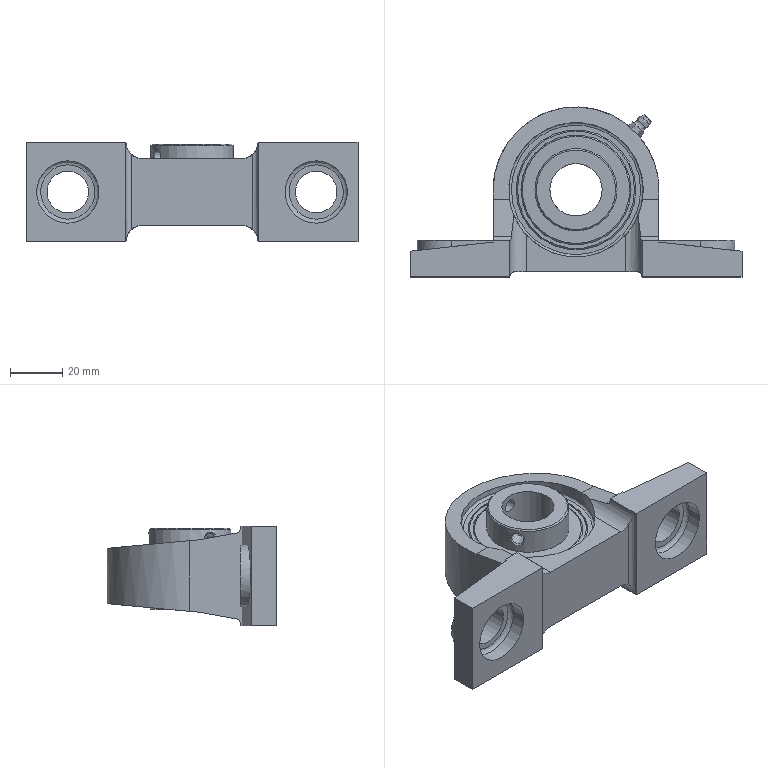Part | STEP file | Pillow block bearing UCP204_D20 | 1 solid | 92 faces | box 127 x 65 x 38 mm | volume 98212 mm3 | plane 48 | cylinder 28 | cone 9 | spline 7 | commonest cylinder face diameters 3.2 x4 12.6 x4 4 x2 4.917 x2 16 x2 23.547 x2